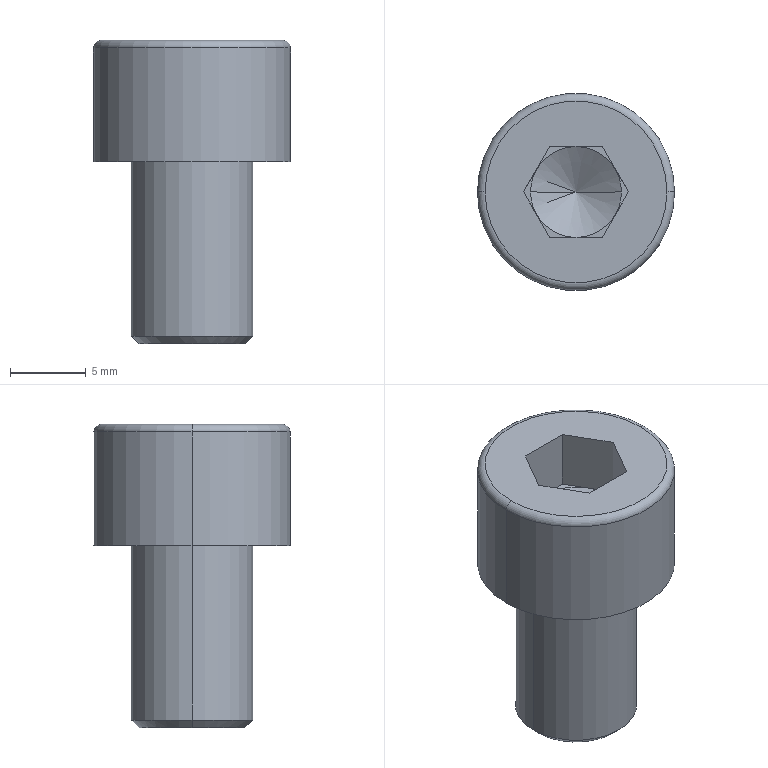Part | NX | features BREP 1 | 1 solid | 25 faces | box 13 x 13 x 20 mm | volume 1519 mm3 | plane 15 | cone 4 | cylinder 4 | torus 2 | commonest cylinder face diameters 8 x2 13 x2
STEP:
#1=CARTESIAN_POINT('',(0.,0.,-5.732));
#2=VERTEX_POINT('',#1);
#3=CARTESIAN_POINT('',(-3.,0.,-4.));
#4=VERTEX_POINT('',#3);
#5=CARTESIAN_POINT('',(-3.,0.,-4.));
#6=DIRECTION('',(-0.866,0.,0.5));
#7=VECTOR('',#6,1000.);
#8=LINE('',#5,#7);
#9=EDGE_CURVE('',#2,#4,#8,.T.);
#10=ORIENTED_EDGE('',*,*,#9,.F.);
#11=CARTESIAN_POINT('',(3.,0.,-4.));
#12=VERTEX_POINT('',#11);
#13=CARTESIAN_POINT('',(3.,0.,-4.));
#14=DIRECTION('',(0.866,0.,0.5));
#15=VECTOR('',#14,1000.);
#16=LINE('',#13,#15);
#17=EDGE_CURVE('',#2,#12,#16,.T.);
#18=ORIENTED_EDGE('',*,*,#17,.T.);
#19=CARTESIAN_POINT('',(2.598,1.5,-4.));
#20=VERTEX_POINT('',#19);
#21=CARTESIAN_POINT('',(0.,0.,-4.));
#22=DIRECTION('',(0.,0.,-1.));
#23=DIRECTION('',(-1.,0.,0.));
#24=AXIS2_PLACEMENT_3D('',#21,#22,#23);
#25=CIRCLE('',#24,3.);
#26=EDGE_CURVE('',#20,#12,#25,.T.);
#27=ORIENTED_EDGE('',*,*,#26,.F.);
#28=CARTESIAN_POINT('',(0.,3.,-4.));
#29=VERTEX_POINT('',#28);
#30=CARTESIAN_POINT('',(0.,0.,-4.));
#31=DIRECTION('',(0.,0.,-1.));
#32=DIRECTION('',(-1.,0.,0.));
#33=AXIS2_PLACEMENT_3D('',#30,#31,#32);
#34=CIRCLE('',#33,3.);
#35=EDGE_CURVE('',#29,#20,#34,.T.);
#36=ORIENTED_EDGE('',*,*,#35,.F.);
#37=CARTESIAN_POINT('',(-2.598,1.5,-4.));
#38=VERTEX_POINT('',#37);
#39=CARTESIAN_POINT('',(0.,0.,-4.));
#40=DIRECTION('',(0.,0.,-1.));
#41=DIRECTION('',(-1.,0.,0.));
#42=AXIS2_PLACEMENT_3D('',#39,#40,#41);
#43=CIRCLE('',#42,3.);
#44=EDGE_CURVE('',#38,#29,#43,.T.);
#45=ORIENTED_EDGE('',*,*,#44,.F.);
#46=CARTESIAN_POINT('',(0.,0.,-4.));
#47=DIRECTION('',(0.,0.,-1.));
#48=DIRECTION('',(-1.,0.,0.));
#49=AXIS2_PLACEMENT_3D('',#46,#47,#48);
#50=CIRCLE('',#49,3.);
#51=EDGE_CURVE('',#4,#38,#50,.T.);
#52=ORIENTED_EDGE('',*,*,#51,.F.);
#53=EDGE_LOOP('',(#10,#18,#27,#36,#45,#52));
#54=FACE_BOUND('',#53,.T.);
#55=CARTESIAN_POINT('',(0.,0.,-4.));
#56=DIRECTION('',(0.,0.,1.));
#57=DIRECTION('',(-1.,0.,0.));
#58=AXIS2_PLACEMENT_3D('',#55,#56,#57);
#59=CONICAL_SURFACE('',#58,3.,1.047);
#60=ADVANCED_FACE('',(#54),#59,.F.);
#61=CARTESIAN_POINT('',(-3.5,0.,-20.));
#62=VERTEX_POINT('',#61);
#63=CARTESIAN_POINT('',(3.5,0.,-20.));
#64=VERTEX_POINT('',#63);
#65=CARTESIAN_POINT('',(0.,0.,-20.));
#66=DIRECTION('',(0.,0.,1.));
#67=DIRECTION('',(1.,0.,0.));
#68=AXIS2_PLACEMENT_3D('',#65,#66,#67);
#69=CIRCLE('',#68,3.5);
#70=EDGE_CURVE('',#62,#64,#69,.T.);
#71=ORIENTED_EDGE('',*,*,#70,.T.);
#72=CARTESIAN_POINT('',(4.,0.,-19.5));
#73=VERTEX_POINT('',#72);
#74=CARTESIAN_POINT('',(3.5,0.,-20.));
#75=DIRECTION('',(0.7071,0.,0.7071));
#76=VECTOR('',#75,1000.);
#77=LINE('',#74,#76);
#78=EDGE_CURVE('',#64,#73,#77,.T.);
#79=ORIENTED_EDGE('',*,*,#78,.T.);
#80=CARTESIAN_POINT('',(-4.,0.,-19.5));
#81=VERTEX_POINT('',#80);
#82=CARTESIAN_POINT('',(0.,0.,-19.5));
#83=DIRECTION('',(0.,0.,-1.));
#84=DIRECTION('',(1.,0.,0.));
#85=AXIS2_PLACEMENT_3D('',#82,#83,#84);
#86=CIRCLE('',#85,4.);
#87=EDGE_CURVE('',#73,#81,#86,.T.);
#88=ORIENTED_EDGE('',*,*,#87,.T.);
#89=CARTESIAN_POINT('',(-3.5,0.,-20.));
#90=DIRECTION('',(-0.7071,0.,0.7071));
#91=VECTOR('',#90,1000.);
#92=LINE('',#89,#91);
#93=EDGE_CURVE('',#62,#81,#92,.T.);
#94=ORIENTED_EDGE('',*,*,#93,.F.);
#95=EDGE_LOOP('',(#71,#79,#88,#94));
#96=FACE_BOUND('',#95,.T.);
#97=CARTESIAN_POINT('',(0.,0.,-20.));
#98=DIRECTION('',(0.,0.,1.));
#99=DIRECTION('',(-1.,0.,0.));
#100=AXIS2_PLACEMENT_3D('',#97,#98,#99);
#101=CONICAL_SURFACE('',#100,3.5,0.7854);
#102=ADVANCED_FACE('',(#96),#101,.T.);
#103=CARTESIAN_POINT('',(6.,0.,0.));
#104=VERTEX_POINT('',#103);
#105=CARTESIAN_POINT('',(-6.,0.,0.));
#106=VERTEX_POINT('',#105);
#107=CARTESIAN_POINT('',(0.,0.,0.));
#108=DIRECTION('',(0.,0.,-1.));
#109=DIRECTION('',(1.,0.,0.));
#110=AXIS2_PLACEMENT_3D('',#107,#108,#109);
#111=CIRCLE('',#110,6.);
#112=EDGE_CURVE('',#104,#106,#111,.T.);
#113=ORIENTED_EDGE('',*,*,#112,.T.);
#114=CARTESIAN_POINT('',(-6.5,0.,-0.5));
#115=VERTEX_POINT('',#114);
#116=CARTESIAN_POINT('',(-6.,0.,-0.5));
#117=DIRECTION('',(0.,-1.,0.));
#118=DIRECTION('',(1.,0.,0.));
#119=AXIS2_PLACEMENT_3D('',#116,#117,#118);
#120=CIRCLE('',#119,0.5);
#121=EDGE_CURVE('',#115,#106,#120,.F.);
#122=ORIENTED_EDGE('',*,*,#121,.F.);
#123=CARTESIAN_POINT('',(6.5,0.,-0.5));
#124=VERTEX_POINT('',#123);
#125=CARTESIAN_POINT('',(0.,0.,-0.5));
#126=DIRECTION('',(0.,0.,1.));
#127=DIRECTION('',(1.,0.,0.));
#128=AXIS2_PLACEMENT_3D('',#125,#126,#127);
#129=CIRCLE('',#128,6.5);
#130=EDGE_CURVE('',#115,#124,#129,.T.);
#131=ORIENTED_EDGE('',*,*,#130,.T.);
#132=CARTESIAN_POINT('',(6.,0.,-0.5));
#133=DIRECTION('',(0.,1.,0.));
#134=DIRECTION('',(0.,0.,1.));
#135=AXIS2_PLACEMENT_3D('',#132,#133,#134);
#136=CIRCLE('',#135,0.5);
#137=EDGE_CURVE('',#124,#104,#136,.F.);
#138=ORIENTED_EDGE('',*,*,#137,.T.);
#139=EDGE_LOOP('',(#113,#122,#131,#138));
#140=FACE_BOUND('',#139,.T.);
#141=CARTESIAN_POINT('',(0.,0.,-0.5));
#142=DIRECTION('',(0.,0.,-1.));
#143=DIRECTION('',(1.,0.,0.));
#144=AXIS2_PLACEMENT_3D('',#141,#142,#143);
#145=TOROIDAL_SURFACE('',#144,6.,0.5);
#146=ADVANCED_FACE('',(#140),#145,.T.);
#147=ORIENTED_EDGE('',*,*,#87,.F.);
#148=CARTESIAN_POINT('',(4.,0.,-8.));
#149=VERTEX_POINT('',#148);
#150=CARTESIAN_POINT('',(4.,0.,-20.));
#151=DIRECTION('',(0.,0.,1.));
#152=VECTOR('',#151,1000.);
#153=LINE('',#150,#152);
#154=EDGE_CURVE('',#73,#149,#153,.T.);
#155=ORIENTED_EDGE('',*,*,#154,.T.);
#156=CARTESIAN_POINT('',(-4.,0.,-8.));
#157=VERTEX_POINT('',#156);
#158=CARTESIAN_POINT('',(0.,0.,-8.));
#159=DIRECTION('',(0.,0.,1.));
#160=DIRECTION('',(1.,0.,0.));
#161=AXIS2_PLACEMENT_3D('',#158,#159,#160);
#162=CIRCLE('',#161,4.);
#163=EDGE_CURVE('',#157,#149,#162,.T.);
#164=ORIENTED_EDGE('',*,*,#163,.F.);
#165=CARTESIAN_POINT('',(-4.,0.,-20.));
#166=DIRECTION('',(0.,0.,1.));
#167=VECTOR('',#166,1000.);
#168=LINE('',#165,#167);
#169=EDGE_CURVE('',#81,#157,#168,.T.);
#170=ORIENTED_EDGE('',*,*,#169,.F.);
#171=EDGE_LOOP('',(#147,#155,#164,#170));
#172=FACE_BOUND('',#171,.T.);
#173=CARTESIAN_POINT('',(0.,0.,-20.));
#174=DIRECTION('',(0.,0.,1.));
#175=DIRECTION('',(-1.,0.,0.));
#176=AXIS2_PLACEMENT_3D('',#173,#174,#175);
#177=CYLINDRICAL_SURFACE('',#176,4.);
#178=ADVANCED_FACE('',(#172),#177,.T.);
#179=CARTESIAN_POINT('',(-6.5,0.,-8.));
#180=VERTEX_POINT('',#179);
#181=CARTESIAN_POINT('',(6.5,0.,-8.));
#182=VERTEX_POINT('',#181);
#183=CARTESIAN_POINT('',(0.,0.,-8.));
#184=DIRECTION('',(0.,0.,1.));
#185=DIRECTION('',(1.,0.,0.));
#186=AXIS2_PLACEMENT_3D('',#183,#184,#185);
#187=CIRCLE('',#186,6.5);
#188=EDGE_CURVE('',#180,#182,#187,.T.);
#189=ORIENTED_EDGE('',*,*,#188,.T.);
#190=CARTESIAN_POINT('',(6.5,0.,-8.));
#191=DIRECTION('',(0.,0.,1.));
#192=VECTOR('',#191,1000.);
#193=LINE('',#190,#192);
#194=EDGE_CURVE('',#182,#124,#193,.T.);
#195=ORIENTED_EDGE('',*,*,#194,.T.);
#196=ORIENTED_EDGE('',*,*,#130,.F.);
#197=CARTESIAN_POINT('',(-6.5,0.,-8.));
#198=DIRECTION('',(0.,0.,1.));
#199=VECTOR('',#198,1000.);
#200=LINE('',#197,#199);
#201=EDGE_CURVE('',#180,#115,#200,.T.);
#202=ORIENTED_EDGE('',*,*,#201,.F.);
#203=EDGE_LOOP('',(#189,#195,#196,#202));
#204=FACE_BOUND('',#203,.T.);
#205=CARTESIAN_POINT('',(0.,0.,-8.));
#206=DIRECTION('',(0.,0.,1.));
#207=DIRECTION('',(-1.,0.,0.));
#208=AXIS2_PLACEMENT_3D('',#205,#206,#207);
#209=CYLINDRICAL_SURFACE('',#208,6.5);
#210=ADVANCED_FACE('',(#204),#209,.T.);
#211=ORIENTED_EDGE('',*,*,#44,.T.);
#212=CARTESIAN_POINT('',(-1.732,3.,-4.));
#213=VERTEX_POINT('',#212);
#214=CARTESIAN_POINT('',(-1.732,3.,-4.));
#215=DIRECTION('',(1.,0.,0.));
#216=VECTOR('',#215,1000.);
#217=LINE('',#214,#216);
#218=EDGE_CURVE('',#213,#29,#217,.T.);
#219=ORIENTED_EDGE('',*,*,#218,.F.);
#220=CARTESIAN_POINT('',(-3.464,0.,-4.));
#221=DIRECTION('',(0.5,0.866,0.));
#222=VECTOR('',#221,1000.);
#223=LINE('',#220,#222);
#224=EDGE_CURVE('',#38,#213,#223,.T.);
#225=ORIENTED_EDGE('',*,*,#224,.F.);
#226=EDGE_LOOP('',(#211,#219,#225));
#227=FACE_BOUND('',#226,.T.);
#228=CARTESIAN_POINT('',(0.,0.,-4.));
#229=DIRECTION('',(0.,0.,1.));
#230=DIRECTION('',(1.,0.,0.));
#231=AXIS2_PLACEMENT_3D('',#228,#229,#230);
#232=PLANE('',#231);
#233=ADVANCED_FACE('',(#227),#232,.T.);
#234=ORIENTED_EDGE('',*,*,#35,.T.);
#235=CARTESIAN_POINT('',(1.732,3.,-4.));
#236=VERTEX_POINT('',#235);
#237=CARTESIAN_POINT('',(1.732,3.,-4.));
#238=DIRECTION('',(0.5,-0.866,0.));
#239=VECTOR('',#238,1000.);
#240=LINE('',#237,#239);
#241=EDGE_CURVE('',#236,#20,#240,.T.);
#242=ORIENTED_EDGE('',*,*,#241,.F.);
#243=CARTESIAN_POINT('',(-1.732,3.,-4.));
#244=DIRECTION('',(1.,0.,0.));
#245=VECTOR('',#244,1000.);
#246=LINE('',#243,#245);
#247=EDGE_CURVE('',#29,#236,#246,.T.);
#248=ORIENTED_EDGE('',*,*,#247,.F.);
#249=EDGE_LOOP('',(#234,#242,#248));
#250=FACE_BOUND('',#249,.T.);
#251=CARTESIAN_POINT('',(0.,0.,-4.));
#252=DIRECTION('',(0.,0.,1.));
#253=DIRECTION('',(1.,0.,0.));
#254=AXIS2_PLACEMENT_3D('',#251,#252,#253);
#255=PLANE('',#254);
#256=ADVANCED_FACE('',(#250),#255,.T.);
#257=ORIENTED_EDGE('',*,*,#26,.T.);
#258=CARTESIAN_POINT('',(2.598,-1.5,-4.));
#259=VERTEX_POINT('',#258);
#260=CARTESIAN_POINT('',(0.,0.,-4.));
#261=DIRECTION('',(0.,0.,-1.));
#262=DIRECTION('',(-1.,0.,0.));
#263=AXIS2_PLACEMENT_3D('',#260,#261,#262);
#264=CIRCLE('',#263,3.);
#265=EDGE_CURVE('',#12,#259,#264,.T.);
#266=ORIENTED_EDGE('',*,*,#265,.T.);
#267=CARTESIAN_POINT('',(3.464,0.,-4.));
#268=VERTEX_POINT('',#267);
#269=CARTESIAN_POINT('',(3.464,0.,-4.));
#270=DIRECTION('',(-0.5,-0.866,0.));
#271=VECTOR('',#270,1000.);
#272=LINE('',#269,#271);
#273=EDGE_CURVE('',#268,#259,#272,.T.);
#274=ORIENTED_EDGE('',*,*,#273,.F.);
#275=CARTESIAN_POINT('',(1.732,3.,-4.));
#276=DIRECTION('',(0.5,-0.866,0.));
#277=VECTOR('',#276,1000.);
#278=LINE('',#275,#277);
#279=EDGE_CURVE('',#20,#268,#278,.T.);
#280=ORIENTED_EDGE('',*,*,#279,.F.);
#281=EDGE_LOOP('',(#257,#266,#274,#280));
#282=FACE_BOUND('',#281,.T.);
#283=CARTESIAN_POINT('',(0.,0.,-4.));
#284=DIRECTION('',(0.,0.,1.));
#285=DIRECTION('',(1.,0.,0.));
#286=AXIS2_PLACEMENT_3D('',#283,#284,#285);
#287=PLANE('',#286);
#288=ADVANCED_FACE('',(#282),#287,.T.);
#289=CARTESIAN_POINT('',(0.,-3.,-4.));
#290=VERTEX_POINT('',#289);
#291=CARTESIAN_POINT('',(0.,0.,-4.));
#292=DIRECTION('',(0.,0.,-1.));
#293=DIRECTION('',(-1.,0.,0.));
#294=AXIS2_PLACEMENT_3D('',#291,#292,#293);
#295=CIRCLE('',#294,3.);
#296=EDGE_CURVE('',#259,#290,#295,.T.);
#297=ORIENTED_EDGE('',*,*,#296,.T.);
#298=CARTESIAN_POINT('',(1.732,-3.,-4.));
#299=VERTEX_POINT('',#298);
#300=CARTESIAN_POINT('',(1.732,-3.,-4.));
#301=DIRECTION('',(-1.,0.,0.));
#302=VECTOR('',#301,1000.);
#303=LINE('',#300,#302);
#304=EDGE_CURVE('',#299,#290,#303,.T.);
#305=ORIENTED_EDGE('',*,*,#304,.F.);
#306=CARTESIAN_POINT('',(3.464,0.,-4.));
#307=DIRECTION('',(-0.5,-0.866,0.));
#308=VECTOR('',#307,1000.);
#309=LINE('',#306,#308);
#310=EDGE_CURVE('',#259,#299,#309,.T.);
#311=ORIENTED_EDGE('',*,*,#310,.F.);
#312=EDGE_LOOP('',(#297,#305,#311));
#313=FACE_BOUND('',#312,.T.);
#314=CARTESIAN_POINT('',(0.,0.,-4.));
#315=DIRECTION('',(0.,0.,1.));
#316=DIRECTION('',(1.,0.,0.));
#317=AXIS2_PLACEMENT_3D('',#314,#315,#316);
#318=PLANE('',#317);
#319=ADVANCED_FACE('',(#313),#318,.T.);
#320=CARTESIAN_POINT('',(-2.598,-1.5,-4.));
#321=VERTEX_POINT('',#320);
#322=CARTESIAN_POINT('',(0.,0.,-4.));
#323=DIRECTION('',(0.,0.,-1.));
#324=DIRECTION('',(-1.,0.,0.));
#325=AXIS2_PLACEMENT_3D('',#322,#323,#324);
#326=CIRCLE('',#325,3.);
#327=EDGE_CURVE('',#290,#321,#326,.T.);
#328=ORIENTED_EDGE('',*,*,#327,.T.);
#329=CARTESIAN_POINT('',(-1.732,-3.,-4.));
#330=VERTEX_POINT('',#329);
#331=CARTESIAN_POINT('',(-1.732,-3.,-4.));
#332=DIRECTION('',(-0.5,0.866,0.));
#333=VECTOR('',#332,1000.);
#334=LINE('',#331,#333);
#335=EDGE_CURVE('',#330,#321,#334,.T.);
#336=ORIENTED_EDGE('',*,*,#335,.F.);
#337=CARTESIAN_POINT('',(1.732,-3.,-4.));
#338=DIRECTION('',(-1.,0.,0.));
#339=VECTOR('',#338,1000.);
#340=LINE('',#337,#339);
#341=EDGE_CURVE('',#290,#330,#340,.T.);
#342=ORIENTED_EDGE('',*,*,#341,.F.);
#343=EDGE_LOOP('',(#328,#336,#342));
#344=FACE_BOUND('',#343,.T.);
#345=CARTESIAN_POINT('',(0.,0.,-4.));
#346=DIRECTION('',(0.,0.,1.));
#347=DIRECTION('',(1.,0.,0.));
#348=AXIS2_PLACEMENT_3D('',#345,#346,#347);
#349=PLANE('',#348);
#350=ADVANCED_FACE('',(#344),#349,.T.);
#351=ORIENTED_EDGE('',*,*,#188,.F.);
#352=CARTESIAN_POINT('',(0.,0.,-8.));
#353=DIRECTION('',(0.,0.,1.));
#354=DIRECTION('',(1.,0.,0.));
#355=AXIS2_PLACEMENT_3D('',#352,#353,#354);
#356=CIRCLE('',#355,6.5);
#357=EDGE_CURVE('',#182,#180,#356,.T.);
#358=ORIENTED_EDGE('',*,*,#357,.F.);
#359=EDGE_LOOP('',(#351,#358));
#360=FACE_BOUND('',#359,.T.);
#361=ORIENTED_EDGE('',*,*,#163,.T.);
#362=CARTESIAN_POINT('',(0.,0.,-8.));
#363=DIRECTION('',(0.,0.,1.));
#364=DIRECTION('',(1.,0.,0.));
#365=AXIS2_PLACEMENT_3D('',#362,#363,#364);
#366=CIRCLE('',#365,4.);
#367=EDGE_CURVE('',#149,#157,#366,.T.);
#368=ORIENTED_EDGE('',*,*,#367,.T.);
#369=EDGE_LOOP('',(#361,#368));
#370=FACE_BOUND('',#369,.T.);
#371=CARTESIAN_POINT('',(0.,0.,-8.));
#372=DIRECTION('',(0.,0.,-1.));
#373=DIRECTION('',(0.,-1.,0.));
#374=AXIS2_PLACEMENT_3D('',#371,#372,#373);
#375=PLANE('',#374);
#376=ADVANCED_FACE('',(#360,#370),#375,.T.);
#377=ORIENTED_EDGE('',*,*,#194,.F.);
#378=ORIENTED_EDGE('',*,*,#357,.T.);
#379=ORIENTED_EDGE('',*,*,#201,.T.);
#380=CARTESIAN_POINT('',(0.,0.,-0.5));
#381=DIRECTION('',(0.,0.,1.));
#382=DIRECTION('',(1.,0.,0.));
#383=AXIS2_PLACEMENT_3D('',#380,#381,#382);
#384=CIRCLE('',#383,6.5);
#385=EDGE_CURVE('',#124,#115,#384,.T.);
#386=ORIENTED_EDGE('',*,*,#385,.F.);
#387=EDGE_LOOP('',(#377,#378,#379,#386));
#388=FACE_BOUND('',#387,.T.);
#389=CARTESIAN_POINT('',(0.,0.,-8.));
#390=DIRECTION('',(0.,0.,1.));
#391=DIRECTION('',(-1.,0.,0.));
#392=AXIS2_PLACEMENT_3D('',#389,#390,#391);
#393=CYLINDRICAL_SURFACE('',#392,6.5);
#394=ADVANCED_FACE('',(#388),#393,.T.);
#395=ORIENTED_EDGE('',*,*,#112,.F.);
#396=CARTESIAN_POINT('',(0.,0.,0.));
#397=DIRECTION('',(0.,0.,-1.));
#398=DIRECTION('',(1.,0.,0.));
#399=AXIS2_PLACEMENT_3D('',#396,#397,#398);
#400=CIRCLE('',#399,6.);
#401=EDGE_CURVE('',#106,#104,#400,.T.);
#402=ORIENTED_EDGE('',*,*,#401,.F.);
#403=EDGE_LOOP('',(#395,#402));
#404=FACE_BOUND('',#403,.T.);
#405=CARTESIAN_POINT('',(-1.732,3.,0.));
#406=VERTEX_POINT('',#405);
#407=CARTESIAN_POINT('',(1.732,3.,0.));
#408=VERTEX_POINT('',#407);
#409=CARTESIAN_POINT('',(-1.732,3.,0.));
#410=DIRECTION('',(1.,0.,0.));
#411=VECTOR('',#410,1000.);
#412=LINE('',#409,#411);
#413=EDGE_CURVE('',#406,#408,#412,.T.);
#414=ORIENTED_EDGE('',*,*,#413,.T.);
#415=CARTESIAN_POINT('',(3.464,0.,0.));
#416=VERTEX_POINT('',#415);
#417=CARTESIAN_POINT('',(1.732,3.,0.));
#418=DIRECTION('',(0.5,-0.866,0.));
#419=VECTOR('',#418,1000.);
#420=LINE('',#417,#419);
#421=EDGE_CURVE('',#408,#416,#420,.T.);
#422=ORIENTED_EDGE('',*,*,#421,.T.);
#423=CARTESIAN_POINT('',(1.732,-3.,0.));
#424=VERTEX_POINT('',#423);
#425=CARTESIAN_POINT('',(3.464,0.,0.));
#426=DIRECTION('',(-0.5,-0.866,0.));
#427=VECTOR('',#426,1000.);
#428=LINE('',#425,#427);
#429=EDGE_CURVE('',#416,#424,#428,.T.);
#430=ORIENTED_EDGE('',*,*,#429,.T.);
#431=CARTESIAN_POINT('',(-1.732,-3.,0.));
#432=VERTEX_POINT('',#431);
#433=CARTESIAN_POINT('',(1.732,-3.,0.));
#434=DIRECTION('',(-1.,0.,0.));
#435=VECTOR('',#434,1000.);
#436=LINE('',#433,#435);
#437=EDGE_CURVE('',#424,#432,#436,.T.);
#438=ORIENTED_EDGE('',*,*,#437,.T.);
#439=CARTESIAN_POINT('',(-3.464,0.,0.));
#440=VERTEX_POINT('',#439);
#441=CARTESIAN_POINT('',(-1.732,-3.,0.));
#442=DIRECTION('',(-0.5,0.866,0.));
#443=VECTOR('',#442,1000.);
#444=LINE('',#441,#443);
#445=EDGE_CURVE('',#432,#440,#444,.T.);
#446=ORIENTED_EDGE('',*,*,#445,.T.);
#447=CARTESIAN_POINT('',(-3.464,0.,0.));
#448=DIRECTION('',(0.5,0.866,0.));
#449=VECTOR('',#448,1000.);
#450=LINE('',#447,#449);
#451=EDGE_CURVE('',#440,#406,#450,.T.);
#452=ORIENTED_EDGE('',*,*,#451,.T.);
#453=EDGE_LOOP('',(#414,#422,#430,#438,#446,#452));
#454=FACE_BOUND('',#453,.T.);
#455=CARTESIAN_POINT('',(0.,0.,0.));
#456=DIRECTION('',(0.,0.,-1.));
#457=DIRECTION('',(0.,-1.,0.));
#458=AXIS2_PLACEMENT_3D('',#455,#456,#457);
#459=PLANE('',#458);
#460=ADVANCED_FACE('',(#404,#454),#459,.F.);
#461=ORIENTED_EDGE('',*,*,#154,.F.);
#462=CARTESIAN_POINT('',(0.,0.,-19.5));
#463=DIRECTION('',(0.,0.,-1.));
#464=DIRECTION('',(1.,0.,0.));
#465=AXIS2_PLACEMENT_3D('',#462,#463,#464);
#466=CIRCLE('',#465,4.);
#467=EDGE_CURVE('',#81,#73,#466,.T.);
#468=ORIENTED_EDGE('',*,*,#467,.F.);
#469=ORIENTED_EDGE('',*,*,#169,.T.);
#470=ORIENTED_EDGE('',*,*,#367,.F.);
#471=EDGE_LOOP('',(#461,#468,#469,#470));
#472=FACE_BOUND('',#471,.T.);
#473=CARTESIAN_POINT('',(0.,0.,-20.));
#474=DIRECTION('',(0.,0.,1.));
#475=DIRECTION('',(-1.,0.,0.));
#476=AXIS2_PLACEMENT_3D('',#473,#474,#475);
#477=CYLINDRICAL_SURFACE('',#476,4.);
#478=ADVANCED_FACE('',(#472),#477,.T.);
#479=ORIENTED_EDGE('',*,*,#70,.F.);
#480=CARTESIAN_POINT('',(0.,0.,-20.));
#481=DIRECTION('',(0.,0.,1.));
#482=DIRECTION('',(1.,0.,0.));
#483=AXIS2_PLACEMENT_3D('',#480,#481,#482);
#484=CIRCLE('',#483,3.5);
#485=EDGE_CURVE('',#64,#62,#484,.T.);
#486=ORIENTED_EDGE('',*,*,#485,.F.);
#487=EDGE_LOOP('',(#479,#486));
#488=FACE_BOUND('',#487,.T.);
#489=CARTESIAN_POINT('',(0.,0.,-20.));
#490=DIRECTION('',(0.,0.,-1.));
#491=DIRECTION('',(0.,-1.,0.));
#492=AXIS2_PLACEMENT_3D('',#489,#490,#491);
#493=PLANE('',#492);
#494=ADVANCED_FACE('',(#488),#493,.T.);
#495=ORIENTED_EDGE('',*,*,#121,.T.);
#496=ORIENTED_EDGE('',*,*,#401,.T.);
#497=ORIENTED_EDGE('',*,*,#137,.F.);
#498=ORIENTED_EDGE('',*,*,#385,.T.);
#499=EDGE_LOOP('',(#495,#496,#497,#498));
#500=FACE_BOUND('',#499,.T.);
#501=CARTESIAN_POINT('',(0.,0.,-0.5));
#502=DIRECTION('',(0.,0.,-1.));
#503=DIRECTION('',(1.,0.,0.));
#504=AXIS2_PLACEMENT_3D('',#501,#502,#503);
#505=TOROIDAL_SURFACE('',#504,6.,0.5);
#506=ADVANCED_FACE('',(#500),#505,.T.);
#507=ORIENTED_EDGE('',*,*,#78,.F.);
#508=ORIENTED_EDGE('',*,*,#485,.T.);
#509=ORIENTED_EDGE('',*,*,#93,.T.);
#510=ORIENTED_EDGE('',*,*,#467,.T.);
#511=EDGE_LOOP('',(#507,#508,#509,#510));
#512=FACE_BOUND('',#511,.T.);
#513=CARTESIAN_POINT('',(0.,0.,-20.));
#514=DIRECTION('',(0.,0.,1.));
#515=DIRECTION('',(-1.,0.,0.));
#516=AXIS2_PLACEMENT_3D('',#513,#514,#515);
#517=CONICAL_SURFACE('',#516,3.5,0.7854);
#518=ADVANCED_FACE('',(#512),#517,.T.);
#519=ORIENTED_EDGE('',*,*,#451,.F.);
#520=CARTESIAN_POINT('',(-3.464,0.,-4.));
#521=VERTEX_POINT('',#520);
#522=CARTESIAN_POINT('',(-3.464,0.,-4.));
#523=DIRECTION('',(0.,0.,1.));
#524=VECTOR('',#523,1000.);
#525=LINE('',#522,#524);
#526=EDGE_CURVE('',#521,#440,#525,.T.);
#527=ORIENTED_EDGE('',*,*,#526,.F.);
#528=CARTESIAN_POINT('',(-3.464,0.,-4.));
#529=DIRECTION('',(0.5,0.866,0.));
#530=VECTOR('',#529,1000.);
#531=LINE('',#528,#530);
#532=EDGE_CURVE('',#521,#38,#531,.T.);
#533=ORIENTED_EDGE('',*,*,#532,.T.);
#534=ORIENTED_EDGE('',*,*,#224,.T.);
#535=CARTESIAN_POINT('',(-1.732,3.,-4.));
#536=DIRECTION('',(0.,0.,1.));
#537=VECTOR('',#536,1000.);
#538=LINE('',#535,#537);
#539=EDGE_CURVE('',#213,#406,#538,.T.);
#540=ORIENTED_EDGE('',*,*,#539,.T.);
#541=EDGE_LOOP('',(#519,#527,#533,#534,#540));
#542=FACE_BOUND('',#541,.T.);
#543=CARTESIAN_POINT('',(-3.464,0.,-4.));
#544=DIRECTION('',(-0.866,0.5,0.));
#545=DIRECTION('',(0.,0.,1.));
#546=AXIS2_PLACEMENT_3D('',#543,#544,#545);
#547=PLANE('',#546);
#548=ADVANCED_FACE('',(#542),#547,.F.);
#549=ORIENTED_EDGE('',*,*,#445,.F.);
#550=CARTESIAN_POINT('',(-1.732,-3.,-4.));
#551=DIRECTION('',(0.,0.,1.));
#552=VECTOR('',#551,1000.);
#553=LINE('',#550,#552);
#554=EDGE_CURVE('',#330,#432,#553,.T.);
#555=ORIENTED_EDGE('',*,*,#554,.F.);
#556=ORIENTED_EDGE('',*,*,#335,.T.);
#557=CARTESIAN_POINT('',(-1.732,-3.,-4.));
#558=DIRECTION('',(-0.5,0.866,0.));
#559=VECTOR('',#558,1000.);
#560=LINE('',#557,#559);
#561=EDGE_CURVE('',#321,#521,#560,.T.);
#562=ORIENTED_EDGE('',*,*,#561,.T.);
#563=ORIENTED_EDGE('',*,*,#526,.T.);
#564=EDGE_LOOP('',(#549,#555,#556,#562,#563));
#565=FACE_BOUND('',#564,.T.);
#566=CARTESIAN_POINT('',(-1.732,-3.,-4.));
#567=DIRECTION('',(-0.866,-0.5,0.));
#568=DIRECTION('',(-0.5,0.866,0.));
#569=AXIS2_PLACEMENT_3D('',#566,#567,#568);
#570=PLANE('',#569);
#571=ADVANCED_FACE('',(#565),#570,.F.);
#572=ORIENTED_EDGE('',*,*,#437,.F.);
#573=CARTESIAN_POINT('',(1.732,-3.,-4.));
#574=DIRECTION('',(0.,0.,1.));
#575=VECTOR('',#574,1000.);
#576=LINE('',#573,#575);
#577=EDGE_CURVE('',#299,#424,#576,.T.);
#578=ORIENTED_EDGE('',*,*,#577,.F.);
#579=ORIENTED_EDGE('',*,*,#304,.T.);
#580=ORIENTED_EDGE('',*,*,#341,.T.);
#581=ORIENTED_EDGE('',*,*,#554,.T.);
#582=EDGE_LOOP('',(#572,#578,#579,#580,#581));
#583=FACE_BOUND('',#582,.T.);
#584=CARTESIAN_POINT('',(1.732,-3.,-4.));
#585=DIRECTION('',(0.,-1.,0.));
#586=DIRECTION('',(0.,0.,-1.));
#587=AXIS2_PLACEMENT_3D('',#584,#585,#586);
#588=PLANE('',#587);
#589=ADVANCED_FACE('',(#583),#588,.F.);
#590=ORIENTED_EDGE('',*,*,#429,.F.);
#591=CARTESIAN_POINT('',(3.464,0.,-4.));
#592=DIRECTION('',(0.,0.,1.));
#593=VECTOR('',#592,1000.);
#594=LINE('',#591,#593);
#595=EDGE_CURVE('',#268,#416,#594,.T.);
#596=ORIENTED_EDGE('',*,*,#595,.F.);
#597=ORIENTED_EDGE('',*,*,#273,.T.);
#598=ORIENTED_EDGE('',*,*,#310,.T.);
#599=ORIENTED_EDGE('',*,*,#577,.T.);
#600=EDGE_LOOP('',(#590,#596,#597,#598,#599));
#601=FACE_BOUND('',#600,.T.);
#602=CARTESIAN_POINT('',(3.464,0.,-4.));
#603=DIRECTION('',(0.866,-0.5,0.));
#604=DIRECTION('',(0.,0.,-1.));
#605=AXIS2_PLACEMENT_3D('',#602,#603,#604);
#606=PLANE('',#605);
#607=ADVANCED_FACE('',(#601),#606,.F.);
#608=ORIENTED_EDGE('',*,*,#421,.F.);
#609=CARTESIAN_POINT('',(1.732,3.,-4.));
#610=DIRECTION('',(0.,0.,1.));
#611=VECTOR('',#610,1000.);
#612=LINE('',#609,#611);
#613=EDGE_CURVE('',#236,#408,#612,.T.);
#614=ORIENTED_EDGE('',*,*,#613,.F.);
#615=ORIENTED_EDGE('',*,*,#241,.T.);
#616=ORIENTED_EDGE('',*,*,#279,.T.);
#617=ORIENTED_EDGE('',*,*,#595,.T.);
#618=EDGE_LOOP('',(#608,#614,#615,#616,#617));
#619=FACE_BOUND('',#618,.T.);
#620=CARTESIAN_POINT('',(1.732,3.,-4.));
#621=DIRECTION('',(0.866,0.5,0.));
#622=DIRECTION('',(0.,0.,-1.));
#623=AXIS2_PLACEMENT_3D('',#620,#621,#622);
#624=PLANE('',#623);
#625=ADVANCED_FACE('',(#619),#624,.F.);
#626=ORIENTED_EDGE('',*,*,#413,.F.);
#627=ORIENTED_EDGE('',*,*,#539,.F.);
#628=ORIENTED_EDGE('',*,*,#218,.T.);
#629=ORIENTED_EDGE('',*,*,#247,.T.);
#630=ORIENTED_EDGE('',*,*,#613,.T.);
#631=EDGE_LOOP('',(#626,#627,#628,#629,#630));
#632=FACE_BOUND('',#631,.T.);
#633=CARTESIAN_POINT('',(-1.732,3.,-4.));
#634=DIRECTION('',(0.,1.,0.));
#635=DIRECTION('',(1.,0.,0.));
#636=AXIS2_PLACEMENT_3D('',#633,#634,#635);
#637=PLANE('',#636);
#638=ADVANCED_FACE('',(#632),#637,.F.);
#639=CARTESIAN_POINT('',(0.,0.,-4.));
#640=DIRECTION('',(0.,0.,-1.));
#641=DIRECTION('',(-1.,0.,0.));
#642=AXIS2_PLACEMENT_3D('',#639,#640,#641);
#643=CIRCLE('',#642,3.);
#644=EDGE_CURVE('',#321,#4,#643,.T.);
#645=ORIENTED_EDGE('',*,*,#644,.T.);
#646=ORIENTED_EDGE('',*,*,#51,.T.);
#647=ORIENTED_EDGE('',*,*,#532,.F.);
#648=ORIENTED_EDGE('',*,*,#561,.F.);
#649=EDGE_LOOP('',(#645,#646,#647,#648));
#650=FACE_BOUND('',#649,.T.);
#651=CARTESIAN_POINT('',(0.,0.,-4.));
#652=DIRECTION('',(0.,0.,1.));
#653=DIRECTION('',(1.,0.,0.));
#654=AXIS2_PLACEMENT_3D('',#651,#652,#653);
#655=PLANE('',#654);
#656=ADVANCED_FACE('',(#650),#655,.T.);
#657=ORIENTED_EDGE('',*,*,#17,.F.);
#658=ORIENTED_EDGE('',*,*,#9,.T.);
#659=ORIENTED_EDGE('',*,*,#644,.F.);
#660=ORIENTED_EDGE('',*,*,#327,.F.);
#661=ORIENTED_EDGE('',*,*,#296,.F.);
#662=ORIENTED_EDGE('',*,*,#265,.F.);
#663=EDGE_LOOP('',(#657,#658,#659,#660,#661,#662));
#664=FACE_BOUND('',#663,.T.);
#665=CARTESIAN_POINT('',(0.,0.,-4.));
#666=DIRECTION('',(0.,0.,1.));
#667=DIRECTION('',(-1.,0.,0.));
#668=AXIS2_PLACEMENT_3D('',#665,#666,#667);
#669=CONICAL_SURFACE('',#668,3.,1.047);
#670=ADVANCED_FACE('',(#664),#669,.F.);
#671=CLOSED_SHELL('',(#60,#102,#146,#178,#210,#233,#256,#288,#319,#350,#376,#394,#460,#478,#494,#506,#518,#548,#571,#589,#607,#625,#638,#656,#670));
#672=MANIFOLD_SOLID_BREP('',#671);
#673=(LENGTH_UNIT()NAMED_UNIT(*)SI_UNIT(.MILLI.,.METRE.));
#674=UNCERTAINTY_MEASURE_WITH_UNIT(LENGTH_MEASURE(0.00001),#673,'','');
#675=(NAMED_UNIT(*)PLANE_ANGLE_UNIT()SI_UNIT($,.RADIAN.));
#676=(NAMED_UNIT(*)SI_UNIT($,.STERADIAN.)SOLID_ANGLE_UNIT());
#677=(GEOMETRIC_REPRESENTATION_CONTEXT(3)GLOBAL_UNCERTAINTY_ASSIGNED_CONTEXT((#674))GLOBAL_UNIT_ASSIGNED_CONTEXT((#673,#675,#676))REPRESENTATION_CONTEXT('',''));
#678=ADVANCED_BREP_SHAPE_REPRESENTATION('',(#672),#677);